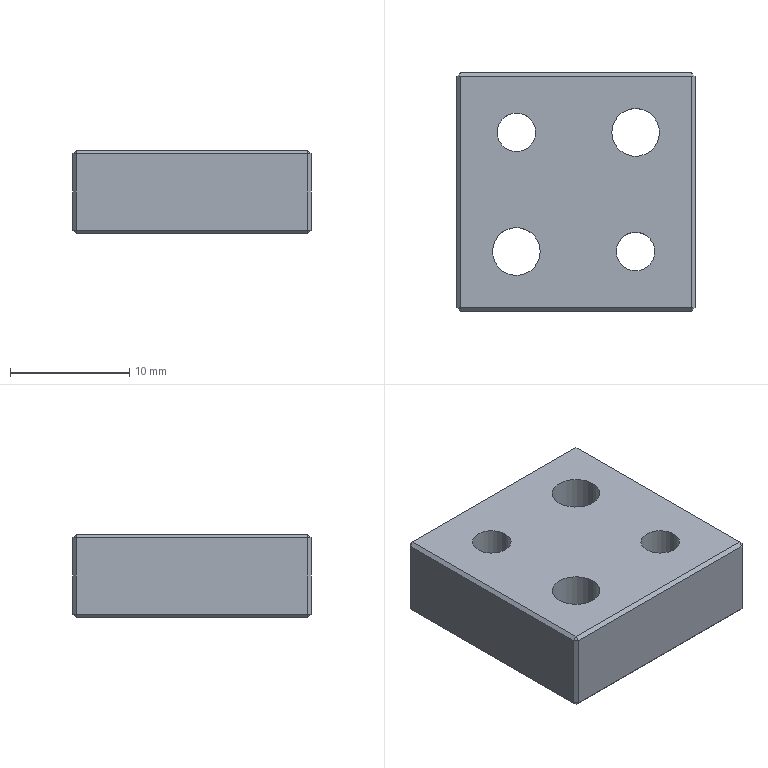Part | STEP file | A037 | 1 solid | 34 faces | box 20 x 20 x 7 mm | volume 2500 mm3 | plane 26 | cylinder 8 | commonest cylinder face diameters 3.242 x4 4 x4